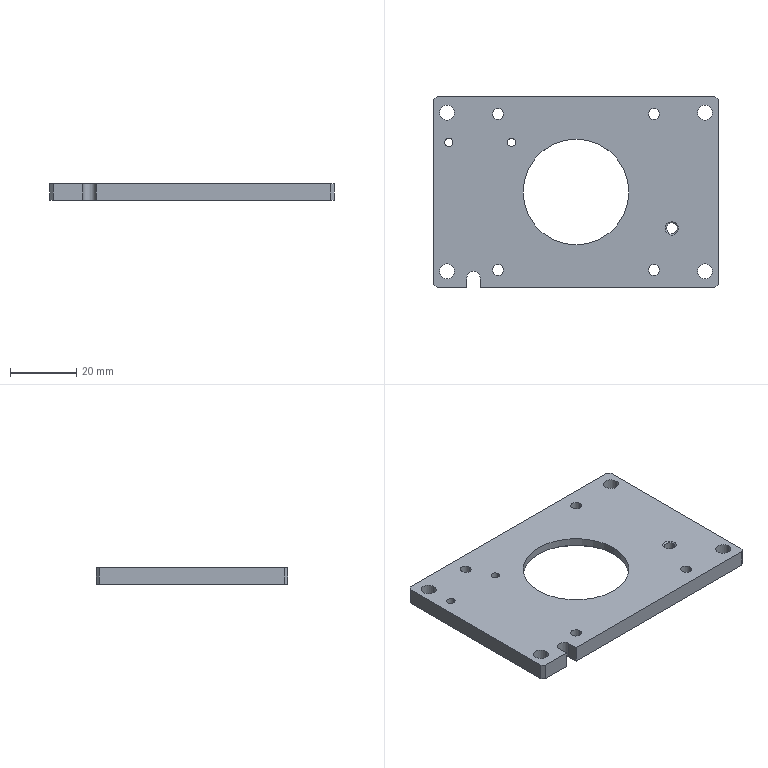Part | SolidWorks | features ICE 5, HoleWzd 4, 3DProfileFeature 2, MirrorPattern 2, Chamfer 1, Cut 1, Extrusion 1, LPattern 1 | 1 solid | 43 faces | box 86 x 58 x 5 mm | volume 19221 mm3 | cylinder 27 | plane 14 | cone 2 | commonest cylinder face diameters 3.3 x10 4.5 x8 2.5 x4 32 x2 39 x2 4 x1
STEP:
#1=CARTESIAN_POINT('',(27.35,-11.,4.625));
#2=VERTEX_POINT('',#1);
#3=CARTESIAN_POINT('',(30.65,-11.,4.625));
#4=VERTEX_POINT('',#3);
#5=CARTESIAN_POINT('',(29.,-11.,4.625));
#6=DIRECTION('',(0.,0.,1.));
#7=DIRECTION('',(1.,0.,0.));
#8=AXIS2_PLACEMENT_3D('',#5,#6,#7);
#9=CIRCLE('',#8,1.65);
#10=EDGE_CURVE('',#2,#4,#9,.T.);
#11=ORIENTED_EDGE('',*,*,#10,.F.);
#12=CARTESIAN_POINT('',(26.975,-11.,5.));
#13=VERTEX_POINT('',#12);
#14=CARTESIAN_POINT('',(26.975,-11.,5.));
#15=DIRECTION('',(-0.7071,0.,0.7071));
#16=VECTOR('',#15,1000.);
#17=LINE('',#14,#16);
#18=EDGE_CURVE('',#2,#13,#17,.T.);
#19=ORIENTED_EDGE('',*,*,#18,.T.);
#20=CARTESIAN_POINT('',(31.025,-11.,5.));
#21=VERTEX_POINT('',#20);
#22=CARTESIAN_POINT('',(29.,-11.,5.));
#23=DIRECTION('',(0.,0.,1.));
#24=DIRECTION('',(1.,0.,0.));
#25=AXIS2_PLACEMENT_3D('',#22,#23,#24);
#26=CIRCLE('',#25,2.025);
#27=EDGE_CURVE('',#13,#21,#26,.T.);
#28=ORIENTED_EDGE('',*,*,#27,.T.);
#29=CARTESIAN_POINT('',(31.025,-11.,5.));
#30=DIRECTION('',(0.7071,0.,0.7071));
#31=VECTOR('',#30,1000.);
#32=LINE('',#29,#31);
#33=EDGE_CURVE('',#4,#21,#32,.T.);
#34=ORIENTED_EDGE('',*,*,#33,.F.);
#35=EDGE_LOOP('',(#11,#19,#28,#34));
#36=FACE_OUTER_BOUND('',#35,.T.);
#37=CARTESIAN_POINT('',(29.,-11.,5.));
#38=DIRECTION('',(0.,0.,1.));
#39=DIRECTION('',(1.,0.,0.));
#40=AXIS2_PLACEMENT_3D('',#37,#38,#39);
#41=CONICAL_SURFACE('',#40,2.025,0.7854);
#42=ADVANCED_FACE('',(#36),#41,.F.);
#43=CARTESIAN_POINT('',(27.35,-11.,0.));
#44=VERTEX_POINT('',#43);
#45=CARTESIAN_POINT('',(30.65,-11.,0.));
#46=VERTEX_POINT('',#45);
#47=CARTESIAN_POINT('',(29.,-11.,0.));
#48=DIRECTION('',(0.,0.,1.));
#49=DIRECTION('',(1.,0.,0.));
#50=AXIS2_PLACEMENT_3D('',#47,#48,#49);
#51=CIRCLE('',#50,1.65);
#52=EDGE_CURVE('',#44,#46,#51,.T.);
#53=ORIENTED_EDGE('',*,*,#52,.F.);
#54=CARTESIAN_POINT('',(27.35,-11.,5.));
#55=DIRECTION('',(0.,0.,1.));
#56=VECTOR('',#55,1000.);
#57=LINE('',#54,#56);
#58=EDGE_CURVE('',#44,#2,#57,.T.);
#59=ORIENTED_EDGE('',*,*,#58,.T.);
#60=ORIENTED_EDGE('',*,*,#10,.T.);
#61=CARTESIAN_POINT('',(30.65,-11.,5.));
#62=DIRECTION('',(0.,0.,1.));
#63=VECTOR('',#62,1000.);
#64=LINE('',#61,#63);
#65=EDGE_CURVE('',#46,#4,#64,.T.);
#66=ORIENTED_EDGE('',*,*,#65,.F.);
#67=EDGE_LOOP('',(#53,#59,#60,#66));
#68=FACE_OUTER_BOUND('',#67,.T.);
#69=CARTESIAN_POINT('',(29.,-11.,5.));
#70=DIRECTION('',(0.,0.,1.));
#71=DIRECTION('',(1.,0.,0.));
#72=AXIS2_PLACEMENT_3D('',#69,#70,#71);
#73=CYLINDRICAL_SURFACE('',#72,1.65);
#74=ADVANCED_FACE('',(#68),#73,.F.);
#75=CARTESIAN_POINT('',(19.5,0.,2.6));
#76=VERTEX_POINT('',#75);
#77=CARTESIAN_POINT('',(-19.5,0.,2.6));
#78=VERTEX_POINT('',#77);
#79=CARTESIAN_POINT('',(0.,0.,2.6));
#80=DIRECTION('',(0.,0.,-1.));
#81=DIRECTION('',(-1.,0.,0.));
#82=AXIS2_PLACEMENT_3D('',#79,#80,#81);
#83=CIRCLE('',#82,19.5);
#84=EDGE_CURVE('',#76,#78,#83,.T.);
#85=ORIENTED_EDGE('',*,*,#84,.F.);
#86=CARTESIAN_POINT('',(19.5,0.,0.));
#87=VERTEX_POINT('',#86);
#88=CARTESIAN_POINT('',(19.5,0.,2.6));
#89=DIRECTION('',(0.,0.,-1.));
#90=VECTOR('',#89,1000.);
#91=LINE('',#88,#90);
#92=EDGE_CURVE('',#76,#87,#91,.T.);
#93=ORIENTED_EDGE('',*,*,#92,.T.);
#94=CARTESIAN_POINT('',(-19.5,0.,0.));
#95=VERTEX_POINT('',#94);
#96=CARTESIAN_POINT('',(0.,0.,0.));
#97=DIRECTION('',(0.,0.,-1.));
#98=DIRECTION('',(-1.,0.,0.));
#99=AXIS2_PLACEMENT_3D('',#96,#97,#98);
#100=CIRCLE('',#99,19.5);
#101=EDGE_CURVE('',#87,#95,#100,.T.);
#102=ORIENTED_EDGE('',*,*,#101,.T.);
#103=CARTESIAN_POINT('',(-19.5,0.,2.6));
#104=DIRECTION('',(0.,0.,-1.));
#105=VECTOR('',#104,1000.);
#106=LINE('',#103,#105);
#107=EDGE_CURVE('',#78,#95,#106,.T.);
#108=ORIENTED_EDGE('',*,*,#107,.F.);
#109=EDGE_LOOP('',(#85,#93,#102,#108));
#110=FACE_OUTER_BOUND('',#109,.T.);
#111=CARTESIAN_POINT('',(0.,0.,2.6));
#112=DIRECTION('',(0.,0.,-1.));
#113=DIRECTION('',(-1.,0.,0.));
#114=AXIS2_PLACEMENT_3D('',#111,#112,#113);
#115=CYLINDRICAL_SURFACE('',#114,19.5);
#116=ADVANCED_FACE('',(#110),#115,.F.);
#117=CARTESIAN_POINT('',(25.22,-23.57,0.));
#118=VERTEX_POINT('',#117);
#119=CARTESIAN_POINT('',(21.92,-23.57,0.));
#120=VERTEX_POINT('',#119);
#121=CARTESIAN_POINT('',(23.57,-23.57,0.));
#122=DIRECTION('',(0.,0.,-1.));
#123=DIRECTION('',(1.,0.,0.));
#124=AXIS2_PLACEMENT_3D('',#121,#122,#123);
#125=CIRCLE('',#124,1.65);
#126=EDGE_CURVE('',#118,#120,#125,.T.);
#127=ORIENTED_EDGE('',*,*,#126,.T.);
#128=CARTESIAN_POINT('',(21.92,-23.57,5.));
#129=VERTEX_POINT('',#128);
#130=CARTESIAN_POINT('',(21.92,-23.57,5.));
#131=DIRECTION('',(0.,0.,1.));
#132=VECTOR('',#131,1000.);
#133=LINE('',#130,#132);
#134=EDGE_CURVE('',#120,#129,#133,.T.);
#135=ORIENTED_EDGE('',*,*,#134,.T.);
#136=CARTESIAN_POINT('',(25.22,-23.57,5.));
#137=VERTEX_POINT('',#136);
#138=CARTESIAN_POINT('',(23.57,-23.57,5.));
#139=DIRECTION('',(0.,0.,1.));
#140=DIRECTION('',(1.,0.,0.));
#141=AXIS2_PLACEMENT_3D('',#138,#139,#140);
#142=CIRCLE('',#141,1.65);
#143=EDGE_CURVE('',#129,#137,#142,.T.);
#144=ORIENTED_EDGE('',*,*,#143,.T.);
#145=CARTESIAN_POINT('',(25.22,-23.57,5.));
#146=DIRECTION('',(0.,0.,1.));
#147=VECTOR('',#146,1000.);
#148=LINE('',#145,#147);
#149=EDGE_CURVE('',#118,#137,#148,.T.);
#150=ORIENTED_EDGE('',*,*,#149,.F.);
#151=EDGE_LOOP('',(#127,#135,#144,#150));
#152=FACE_OUTER_BOUND('',#151,.T.);
#153=CARTESIAN_POINT('',(23.57,-23.57,5.));
#154=DIRECTION('',(0.,0.,1.));
#155=DIRECTION('',(1.,0.,0.));
#156=AXIS2_PLACEMENT_3D('',#153,#154,#155);
#157=CYLINDRICAL_SURFACE('',#156,1.65);
#158=ADVANCED_FACE('',(#152),#157,.F.);
#159=CARTESIAN_POINT('',(25.22,23.57,0.));
#160=VERTEX_POINT('',#159);
#161=CARTESIAN_POINT('',(21.92,23.57,0.));
#162=VERTEX_POINT('',#161);
#163=CARTESIAN_POINT('',(23.57,23.57,0.));
#164=DIRECTION('',(0.,0.,-1.));
#165=DIRECTION('',(1.,0.,0.));
#166=AXIS2_PLACEMENT_3D('',#163,#164,#165);
#167=CIRCLE('',#166,1.65);
#168=EDGE_CURVE('',#160,#162,#167,.T.);
#169=ORIENTED_EDGE('',*,*,#168,.T.);
#170=CARTESIAN_POINT('',(21.92,23.57,5.));
#171=VERTEX_POINT('',#170);
#172=CARTESIAN_POINT('',(21.92,23.57,5.));
#173=DIRECTION('',(0.,0.,1.));
#174=VECTOR('',#173,1000.);
#175=LINE('',#172,#174);
#176=EDGE_CURVE('',#162,#171,#175,.T.);
#177=ORIENTED_EDGE('',*,*,#176,.T.);
#178=CARTESIAN_POINT('',(25.22,23.57,5.));
#179=VERTEX_POINT('',#178);
#180=CARTESIAN_POINT('',(23.57,23.57,5.));
#181=DIRECTION('',(0.,0.,1.));
#182=DIRECTION('',(1.,0.,0.));
#183=AXIS2_PLACEMENT_3D('',#180,#181,#182);
#184=CIRCLE('',#183,1.65);
#185=EDGE_CURVE('',#171,#179,#184,.T.);
#186=ORIENTED_EDGE('',*,*,#185,.T.);
#187=CARTESIAN_POINT('',(25.22,23.57,5.));
#188=DIRECTION('',(0.,0.,1.));
#189=VECTOR('',#188,1000.);
#190=LINE('',#187,#189);
#191=EDGE_CURVE('',#160,#179,#190,.T.);
#192=ORIENTED_EDGE('',*,*,#191,.F.);
#193=EDGE_LOOP('',(#169,#177,#186,#192));
#194=FACE_OUTER_BOUND('',#193,.T.);
#195=CARTESIAN_POINT('',(23.57,23.57,5.));
#196=DIRECTION('',(0.,0.,1.));
#197=DIRECTION('',(1.,0.,0.));
#198=AXIS2_PLACEMENT_3D('',#195,#196,#197);
#199=CYLINDRICAL_SURFACE('',#198,1.65);
#200=ADVANCED_FACE('',(#194),#199,.F.);
#201=CARTESIAN_POINT('',(-21.92,-23.57,0.));
#202=VERTEX_POINT('',#201);
#203=CARTESIAN_POINT('',(-25.22,-23.57,0.));
#204=VERTEX_POINT('',#203);
#205=CARTESIAN_POINT('',(-23.57,-23.57,0.));
#206=DIRECTION('',(0.,0.,-1.));
#207=DIRECTION('',(1.,0.,0.));
#208=AXIS2_PLACEMENT_3D('',#205,#206,#207);
#209=CIRCLE('',#208,1.65);
#210=EDGE_CURVE('',#202,#204,#209,.T.);
#211=ORIENTED_EDGE('',*,*,#210,.T.);
#212=CARTESIAN_POINT('',(-25.22,-23.57,5.));
#213=VERTEX_POINT('',#212);
#214=CARTESIAN_POINT('',(-25.22,-23.57,5.));
#215=DIRECTION('',(0.,0.,1.));
#216=VECTOR('',#215,1000.);
#217=LINE('',#214,#216);
#218=EDGE_CURVE('',#204,#213,#217,.T.);
#219=ORIENTED_EDGE('',*,*,#218,.T.);
#220=CARTESIAN_POINT('',(-21.92,-23.57,5.));
#221=VERTEX_POINT('',#220);
#222=CARTESIAN_POINT('',(-23.57,-23.57,5.));
#223=DIRECTION('',(0.,0.,1.));
#224=DIRECTION('',(1.,0.,0.));
#225=AXIS2_PLACEMENT_3D('',#222,#223,#224);
#226=CIRCLE('',#225,1.65);
#227=EDGE_CURVE('',#213,#221,#226,.T.);
#228=ORIENTED_EDGE('',*,*,#227,.T.);
#229=CARTESIAN_POINT('',(-21.92,-23.57,5.));
#230=DIRECTION('',(0.,0.,1.));
#231=VECTOR('',#230,1000.);
#232=LINE('',#229,#231);
#233=EDGE_CURVE('',#202,#221,#232,.T.);
#234=ORIENTED_EDGE('',*,*,#233,.F.);
#235=EDGE_LOOP('',(#211,#219,#228,#234));
#236=FACE_OUTER_BOUND('',#235,.T.);
#237=CARTESIAN_POINT('',(-23.57,-23.57,5.));
#238=DIRECTION('',(0.,0.,1.));
#239=DIRECTION('',(1.,0.,0.));
#240=AXIS2_PLACEMENT_3D('',#237,#238,#239);
#241=CYLINDRICAL_SURFACE('',#240,1.65);
#242=ADVANCED_FACE('',(#236),#241,.F.);
#243=CARTESIAN_POINT('',(-21.92,23.57,0.));
#244=VERTEX_POINT('',#243);
#245=CARTESIAN_POINT('',(-25.22,23.57,0.));
#246=VERTEX_POINT('',#245);
#247=CARTESIAN_POINT('',(-23.57,23.57,0.));
#248=DIRECTION('',(0.,0.,-1.));
#249=DIRECTION('',(1.,0.,0.));
#250=AXIS2_PLACEMENT_3D('',#247,#248,#249);
#251=CIRCLE('',#250,1.65);
#252=EDGE_CURVE('',#244,#246,#251,.T.);
#253=ORIENTED_EDGE('',*,*,#252,.T.);
#254=CARTESIAN_POINT('',(-25.22,23.57,5.));
#255=VERTEX_POINT('',#254);
#256=CARTESIAN_POINT('',(-25.22,23.57,5.));
#257=DIRECTION('',(0.,0.,1.));
#258=VECTOR('',#257,1000.);
#259=LINE('',#256,#258);
#260=EDGE_CURVE('',#246,#255,#259,.T.);
#261=ORIENTED_EDGE('',*,*,#260,.T.);
#262=CARTESIAN_POINT('',(-21.92,23.57,5.));
#263=VERTEX_POINT('',#262);
#264=CARTESIAN_POINT('',(-23.57,23.57,5.));
#265=DIRECTION('',(0.,0.,1.));
#266=DIRECTION('',(1.,0.,0.));
#267=AXIS2_PLACEMENT_3D('',#264,#265,#266);
#268=CIRCLE('',#267,1.65);
#269=EDGE_CURVE('',#255,#263,#268,.T.);
#270=ORIENTED_EDGE('',*,*,#269,.T.);
#271=CARTESIAN_POINT('',(-21.92,23.57,5.));
#272=DIRECTION('',(0.,0.,1.));
#273=VECTOR('',#272,1000.);
#274=LINE('',#271,#273);
#275=EDGE_CURVE('',#244,#263,#274,.T.);
#276=ORIENTED_EDGE('',*,*,#275,.F.);
#277=EDGE_LOOP('',(#253,#261,#270,#276));
#278=FACE_OUTER_BOUND('',#277,.T.);
#279=CARTESIAN_POINT('',(-23.57,23.57,5.));
#280=DIRECTION('',(0.,0.,1.));
#281=DIRECTION('',(1.,0.,0.));
#282=AXIS2_PLACEMENT_3D('',#279,#280,#281);
#283=CYLINDRICAL_SURFACE('',#282,1.65);
#284=ADVANCED_FACE('',(#278),#283,.F.);
#285=CARTESIAN_POINT('',(-37.25,15.,0.));
#286=VERTEX_POINT('',#285);
#287=CARTESIAN_POINT('',(-39.75,15.,0.));
#288=VERTEX_POINT('',#287);
#289=CARTESIAN_POINT('',(-38.5,15.,0.));
#290=DIRECTION('',(0.,0.,-1.));
#291=DIRECTION('',(1.,0.,0.));
#292=AXIS2_PLACEMENT_3D('',#289,#290,#291);
#293=CIRCLE('',#292,1.25);
#294=EDGE_CURVE('',#286,#288,#293,.T.);
#295=ORIENTED_EDGE('',*,*,#294,.T.);
#296=CARTESIAN_POINT('',(-39.75,15.,5.));
#297=VERTEX_POINT('',#296);
#298=CARTESIAN_POINT('',(-39.75,15.,5.));
#299=DIRECTION('',(0.,0.,1.));
#300=VECTOR('',#299,1000.);
#301=LINE('',#298,#300);
#302=EDGE_CURVE('',#288,#297,#301,.T.);
#303=ORIENTED_EDGE('',*,*,#302,.T.);
#304=CARTESIAN_POINT('',(-37.25,15.,5.));
#305=VERTEX_POINT('',#304);
#306=CARTESIAN_POINT('',(-38.5,15.,5.));
#307=DIRECTION('',(0.,0.,1.));
#308=DIRECTION('',(1.,0.,0.));
#309=AXIS2_PLACEMENT_3D('',#306,#307,#308);
#310=CIRCLE('',#309,1.25);
#311=EDGE_CURVE('',#297,#305,#310,.T.);
#312=ORIENTED_EDGE('',*,*,#311,.T.);
#313=CARTESIAN_POINT('',(-37.25,15.,5.));
#314=DIRECTION('',(0.,0.,1.));
#315=VECTOR('',#314,1000.);
#316=LINE('',#313,#315);
#317=EDGE_CURVE('',#286,#305,#316,.T.);
#318=ORIENTED_EDGE('',*,*,#317,.F.);
#319=EDGE_LOOP('',(#295,#303,#312,#318));
#320=FACE_OUTER_BOUND('',#319,.T.);
#321=CARTESIAN_POINT('',(-38.5,15.,5.));
#322=DIRECTION('',(0.,0.,1.));
#323=DIRECTION('',(1.,0.,0.));
#324=AXIS2_PLACEMENT_3D('',#321,#322,#323);
#325=CYLINDRICAL_SURFACE('',#324,1.25);
#326=ADVANCED_FACE('',(#320),#325,.F.);
#327=CARTESIAN_POINT('',(-18.25,15.,0.));
#328=VERTEX_POINT('',#327);
#329=CARTESIAN_POINT('',(-20.75,15.,0.));
#330=VERTEX_POINT('',#329);
#331=CARTESIAN_POINT('',(-19.5,15.,0.));
#332=DIRECTION('',(0.,0.,-1.));
#333=DIRECTION('',(1.,0.,0.));
#334=AXIS2_PLACEMENT_3D('',#331,#332,#333);
#335=CIRCLE('',#334,1.25);
#336=EDGE_CURVE('',#328,#330,#335,.T.);
#337=ORIENTED_EDGE('',*,*,#336,.T.);
#338=CARTESIAN_POINT('',(-20.75,15.,5.));
#339=VERTEX_POINT('',#338);
#340=CARTESIAN_POINT('',(-20.75,15.,5.));
#341=DIRECTION('',(0.,0.,1.));
#342=VECTOR('',#341,1000.);
#343=LINE('',#340,#342);
#344=EDGE_CURVE('',#330,#339,#343,.T.);
#345=ORIENTED_EDGE('',*,*,#344,.T.);
#346=CARTESIAN_POINT('',(-18.25,15.,5.));
#347=VERTEX_POINT('',#346);
#348=CARTESIAN_POINT('',(-19.5,15.,5.));
#349=DIRECTION('',(0.,0.,1.));
#350=DIRECTION('',(1.,0.,0.));
#351=AXIS2_PLACEMENT_3D('',#348,#349,#350);
#352=CIRCLE('',#351,1.25);
#353=EDGE_CURVE('',#339,#347,#352,.T.);
#354=ORIENTED_EDGE('',*,*,#353,.T.);
#355=CARTESIAN_POINT('',(-18.25,15.,5.));
#356=DIRECTION('',(0.,0.,1.));
#357=VECTOR('',#356,1000.);
#358=LINE('',#355,#357);
#359=EDGE_CURVE('',#328,#347,#358,.T.);
#360=ORIENTED_EDGE('',*,*,#359,.F.);
#361=EDGE_LOOP('',(#337,#345,#354,#360));
#362=FACE_OUTER_BOUND('',#361,.T.);
#363=CARTESIAN_POINT('',(-19.5,15.,5.));
#364=DIRECTION('',(0.,0.,1.));
#365=DIRECTION('',(1.,0.,0.));
#366=AXIS2_PLACEMENT_3D('',#363,#364,#365);
#367=CYLINDRICAL_SURFACE('',#366,1.25);
#368=ADVANCED_FACE('',(#362),#367,.F.);
#369=CARTESIAN_POINT('',(-41.25,-24.,5.));
#370=VERTEX_POINT('',#369);
#371=CARTESIAN_POINT('',(-36.75,-24.,5.));
#372=VERTEX_POINT('',#371);
#373=CARTESIAN_POINT('',(-39.,-24.,5.));
#374=DIRECTION('',(0.,0.,1.));
#375=DIRECTION('',(-1.,0.,0.));
#376=AXIS2_PLACEMENT_3D('',#373,#374,#375);
#377=CIRCLE('',#376,2.25);
#378=EDGE_CURVE('',#370,#372,#377,.T.);
#379=ORIENTED_EDGE('',*,*,#378,.T.);
#380=CARTESIAN_POINT('',(-36.75,-24.,0.));
#381=VERTEX_POINT('',#380);
#382=CARTESIAN_POINT('',(-36.75,-24.,5.));
#383=DIRECTION('',(0.,0.,-1.));
#384=VECTOR('',#383,1000.);
#385=LINE('',#382,#384);
#386=EDGE_CURVE('',#372,#381,#385,.T.);
#387=ORIENTED_EDGE('',*,*,#386,.T.);
#388=CARTESIAN_POINT('',(-41.25,-24.,0.));
#389=VERTEX_POINT('',#388);
#390=CARTESIAN_POINT('',(-39.,-24.,0.));
#391=DIRECTION('',(0.,0.,1.));
#392=DIRECTION('',(1.,0.,0.));
#393=AXIS2_PLACEMENT_3D('',#390,#391,#392);
#394=CIRCLE('',#393,2.25);
#395=EDGE_CURVE('',#389,#381,#394,.T.);
#396=ORIENTED_EDGE('',*,*,#395,.F.);
#397=CARTESIAN_POINT('',(-41.25,-24.,5.));
#398=DIRECTION('',(0.,0.,-1.));
#399=VECTOR('',#398,1000.);
#400=LINE('',#397,#399);
#401=EDGE_CURVE('',#370,#389,#400,.T.);
#402=ORIENTED_EDGE('',*,*,#401,.F.);
#403=EDGE_LOOP('',(#379,#387,#396,#402));
#404=FACE_OUTER_BOUND('',#403,.T.);
#405=CARTESIAN_POINT('',(-39.,-24.,5.));
#406=DIRECTION('',(0.,0.,-1.));
#407=DIRECTION('',(-1.,0.,0.));
#408=AXIS2_PLACEMENT_3D('',#405,#406,#407);
#409=CYLINDRICAL_SURFACE('',#408,2.25);
#410=ADVANCED_FACE('',(#404),#409,.F.);
#411=CARTESIAN_POINT('',(36.75,-24.,5.));
#412=VERTEX_POINT('',#411);
#413=CARTESIAN_POINT('',(41.25,-24.,5.));
#414=VERTEX_POINT('',#413);
#415=CARTESIAN_POINT('',(39.,-24.,5.));
#416=DIRECTION('',(0.,0.,1.));
#417=DIRECTION('',(1.,0.,0.));
#418=AXIS2_PLACEMENT_3D('',#415,#416,#417);
#419=CIRCLE('',#418,2.25);
#420=EDGE_CURVE('',#412,#414,#419,.T.);
#421=ORIENTED_EDGE('',*,*,#420,.T.);
#422=CARTESIAN_POINT('',(41.25,-24.,0.));
#423=VERTEX_POINT('',#422);
#424=CARTESIAN_POINT('',(41.25,-24.,5.));
#425=DIRECTION('',(0.,0.,-1.));
#426=VECTOR('',#425,1000.);
#427=LINE('',#424,#426);
#428=EDGE_CURVE('',#414,#423,#427,.T.);
#429=ORIENTED_EDGE('',*,*,#428,.T.);
#430=CARTESIAN_POINT('',(36.75,-24.,0.));
#431=VERTEX_POINT('',#430);
#432=CARTESIAN_POINT('',(39.,-24.,0.));
#433=DIRECTION('',(0.,0.,1.));
#434=DIRECTION('',(1.,0.,0.));
#435=AXIS2_PLACEMENT_3D('',#432,#433,#434);
#436=CIRCLE('',#435,2.25);
#437=EDGE_CURVE('',#431,#423,#436,.T.);
#438=ORIENTED_EDGE('',*,*,#437,.F.);
#439=CARTESIAN_POINT('',(36.75,-24.,5.));
#440=DIRECTION('',(0.,0.,-1.));
#441=VECTOR('',#440,1000.);
#442=LINE('',#439,#441);
#443=EDGE_CURVE('',#412,#431,#442,.T.);
#444=ORIENTED_EDGE('',*,*,#443,.F.);
#445=EDGE_LOOP('',(#421,#429,#438,#444));
#446=FACE_OUTER_BOUND('',#445,.T.);
#447=CARTESIAN_POINT('',(39.,-24.,5.));
#448=DIRECTION('',(0.,0.,-1.));
#449=DIRECTION('',(-1.,0.,0.));
#450=AXIS2_PLACEMENT_3D('',#447,#448,#449);
#451=CYLINDRICAL_SURFACE('',#450,2.25);
#452=ADVANCED_FACE('',(#446),#451,.F.);
#453=CARTESIAN_POINT('',(36.75,24.,5.));
#454=VERTEX_POINT('',#453);
#455=CARTESIAN_POINT('',(41.25,24.,5.));
#456=VERTEX_POINT('',#455);
#457=CARTESIAN_POINT('',(39.,24.,5.));
#458=DIRECTION('',(0.,0.,1.));
#459=DIRECTION('',(-1.,0.,0.));
#460=AXIS2_PLACEMENT_3D('',#457,#458,#459);
#461=CIRCLE('',#460,2.25);
#462=EDGE_CURVE('',#454,#456,#461,.T.);
#463=ORIENTED_EDGE('',*,*,#462,.T.);
#464=CARTESIAN_POINT('',(41.25,24.,0.));
#465=VERTEX_POINT('',#464);
#466=CARTESIAN_POINT('',(41.25,24.,5.));
#467=DIRECTION('',(0.,0.,-1.));
#468=VECTOR('',#467,1000.);
#469=LINE('',#466,#468);
#470=EDGE_CURVE('',#456,#465,#469,.T.);
#471=ORIENTED_EDGE('',*,*,#470,.T.);
#472=CARTESIAN_POINT('',(36.75,24.,0.));
#473=VERTEX_POINT('',#472);
#474=CARTESIAN_POINT('',(39.,24.,0.));
#475=DIRECTION('',(0.,0.,1.));
#476=DIRECTION('',(1.,0.,0.));
#477=AXIS2_PLACEMENT_3D('',#474,#475,#476);
#478=CIRCLE('',#477,2.25);
#479=EDGE_CURVE('',#473,#465,#478,.T.);
#480=ORIENTED_EDGE('',*,*,#479,.F.);
#481=CARTESIAN_POINT('',(36.75,24.,5.));
#482=DIRECTION('',(0.,0.,-1.));
#483=VECTOR('',#482,1000.);
#484=LINE('',#481,#483);
#485=EDGE_CURVE('',#454,#473,#484,.T.);
#486=ORIENTED_EDGE('',*,*,#485,.F.);
#487=EDGE_LOOP('',(#463,#471,#480,#486));
#488=FACE_OUTER_BOUND('',#487,.T.);
#489=CARTESIAN_POINT('',(39.,24.,5.));
#490=DIRECTION('',(0.,0.,-1.));
#491=DIRECTION('',(-1.,0.,0.));
#492=AXIS2_PLACEMENT_3D('',#489,#490,#491);
#493=CYLINDRICAL_SURFACE('',#492,2.25);
#494=ADVANCED_FACE('',(#488),#493,.F.);
#495=CARTESIAN_POINT('',(-41.25,24.,5.));
#496=VERTEX_POINT('',#495);
#497=CARTESIAN_POINT('',(-36.75,24.,5.));
#498=VERTEX_POINT('',#497);
#499=CARTESIAN_POINT('',(-39.,24.,5.));
#500=DIRECTION('',(0.,0.,1.));
#501=DIRECTION('',(1.,0.,0.));
#502=AXIS2_PLACEMENT_3D('',#499,#500,#501);
#503=CIRCLE('',#502,2.25);
#504=EDGE_CURVE('',#496,#498,#503,.T.);
#505=ORIENTED_EDGE('',*,*,#504,.T.);
#506=CARTESIAN_POINT('',(-36.75,24.,0.));
#507=VERTEX_POINT('',#506);
#508=CARTESIAN_POINT('',(-36.75,24.,5.));
#509=DIRECTION('',(0.,0.,-1.));
#510=VECTOR('',#509,1000.);
#511=LINE('',#508,#510);
#512=EDGE_CURVE('',#498,#507,#511,.T.);
#513=ORIENTED_EDGE('',*,*,#512,.T.);
#514=CARTESIAN_POINT('',(-41.25,24.,0.));
#515=VERTEX_POINT('',#514);
#516=CARTESIAN_POINT('',(-39.,24.,0.));
#517=DIRECTION('',(0.,0.,1.));
#518=DIRECTION('',(1.,0.,0.));
#519=AXIS2_PLACEMENT_3D('',#516,#517,#518);
#520=CIRCLE('',#519,2.25);
#521=EDGE_CURVE('',#515,#507,#520,.T.);
#522=ORIENTED_EDGE('',*,*,#521,.F.);
#523=CARTESIAN_POINT('',(-41.25,24.,5.));
#524=DIRECTION('',(0.,0.,-1.));
#525=VECTOR('',#524,1000.);
#526=LINE('',#523,#525);
#527=EDGE_CURVE('',#496,#515,#526,.T.);
#528=ORIENTED_EDGE('',*,*,#527,.F.);
#529=EDGE_LOOP('',(#505,#513,#522,#528));
#530=FACE_OUTER_BOUND('',#529,.T.);
#531=CARTESIAN_POINT('',(-39.,24.,5.));
#532=DIRECTION('',(0.,0.,-1.));
#533=DIRECTION('',(-1.,0.,0.));
#534=AXIS2_PLACEMENT_3D('',#531,#532,#533);
#535=CYLINDRICAL_SURFACE('',#534,2.25);
#536=ADVANCED_FACE('',(#530),#535,.F.);
#537=CARTESIAN_POINT('',(-16.,0.,5.));
#538=VERTEX_POINT('',#537);
#539=CARTESIAN_POINT('',(16.,0.,5.));
#540=VERTEX_POINT('',#539);
#541=CARTESIAN_POINT('',(0.,0.,5.));
#542=DIRECTION('',(0.,0.,1.));
#543=DIRECTION('',(1.,0.,0.));
#544=AXIS2_PLACEMENT_3D('',#541,#542,#543);
#545=CIRCLE('',#544,16.);
#546=EDGE_CURVE('',#538,#540,#545,.T.);
#547=ORIENTED_EDGE('',*,*,#546,.T.);
#548=CARTESIAN_POINT('',(16.,0.,2.6));
#549=VERTEX_POINT('',#548);
#550=CARTESIAN_POINT('',(16.,0.,5.));
#551=DIRECTION('',(0.,0.,-1.));
#552=VECTOR('',#551,1000.);
#553=LINE('',#550,#552);
#554=EDGE_CURVE('',#540,#549,#553,.T.);
#555=ORIENTED_EDGE('',*,*,#554,.T.);
#556=CARTESIAN_POINT('',(-16.,0.,2.6));
#557=VERTEX_POINT('',#556);
#558=CARTESIAN_POINT('',(0.,0.,2.6));
#559=DIRECTION('',(0.,0.,-1.));
#560=DIRECTION('',(-1.,0.,0.));
#561=AXIS2_PLACEMENT_3D('',#558,#559,#560);
#562=CIRCLE('',#561,16.);
#563=EDGE_CURVE('',#549,#557,#562,.T.);
#564=ORIENTED_EDGE('',*,*,#563,.T.);
#565=CARTESIAN_POINT('',(-16.,0.,5.));
#566=DIRECTION('',(0.,0.,-1.));
#567=VECTOR('',#566,1000.);
#568=LINE('',#565,#567);
#569=EDGE_CURVE('',#538,#557,#568,.T.);
#570=ORIENTED_EDGE('',*,*,#569,.F.);
#571=EDGE_LOOP('',(#547,#555,#564,#570));
#572=FACE_OUTER_BOUND('',#571,.T.);
#573=CARTESIAN_POINT('',(0.,0.,5.));
#574=DIRECTION('',(0.,0.,-1.));
#575=DIRECTION('',(-1.,0.,0.));
#576=AXIS2_PLACEMENT_3D('',#573,#574,#575);
#577=CYLINDRICAL_SURFACE('',#576,16.);
#578=ADVANCED_FACE('',(#572),#577,.F.);
#579=ORIENTED_EDGE('',*,*,#554,.F.);
#580=CARTESIAN_POINT('',(0.,0.,5.));
#581=DIRECTION('',(0.,0.,1.));
#582=DIRECTION('',(1.,0.,0.));
#583=AXIS2_PLACEMENT_3D('',#580,#581,#582);
#584=CIRCLE('',#583,16.);
#585=EDGE_CURVE('',#540,#538,#584,.T.);
#586=ORIENTED_EDGE('',*,*,#585,.T.);
#587=ORIENTED_EDGE('',*,*,#569,.T.);
#588=CARTESIAN_POINT('',(0.,0.,2.6));
#589=DIRECTION('',(0.,0.,-1.));
#590=DIRECTION('',(-1.,0.,0.));
#591=AXIS2_PLACEMENT_3D('',#588,#589,#590);
#592=CIRCLE('',#591,16.);
#593=EDGE_CURVE('',#557,#549,#592,.T.);
#594=ORIENTED_EDGE('',*,*,#593,.T.);
#595=EDGE_LOOP('',(#579,#586,#587,#594));
#596=FACE_OUTER_BOUND('',#595,.T.);
#597=CARTESIAN_POINT('',(0.,0.,5.));
#598=DIRECTION('',(0.,0.,-1.));
#599=DIRECTION('',(-1.,0.,0.));
#600=AXIS2_PLACEMENT_3D('',#597,#598,#599);
#601=CYLINDRICAL_SURFACE('',#600,16.);
#602=ADVANCED_FACE('',(#596),#601,.F.);
#603=CARTESIAN_POINT('',(-42.,-29.,5.));
#604=VERTEX_POINT('',#603);
#605=CARTESIAN_POINT('',(-42.,-29.,0.));
#606=VERTEX_POINT('',#605);
#607=CARTESIAN_POINT('',(-42.,-29.,5.));
#608=DIRECTION('',(0.,0.,-1.));
#609=VECTOR('',#608,1000.);
#610=LINE('',#607,#609);
#611=EDGE_CURVE('',#604,#606,#610,.T.);
#612=ORIENTED_EDGE('',*,*,#611,.T.);
#613=CARTESIAN_POINT('',(-33.,-29.,0.));
#614=VERTEX_POINT('',#613);
#615=CARTESIAN_POINT('',(160.212,-29.,0.));
#616=DIRECTION('',(1.,0.,0.));
#617=VECTOR('',#616,1000.);
#618=LINE('',#615,#617);
#619=EDGE_CURVE('',#606,#614,#618,.T.);
#620=ORIENTED_EDGE('',*,*,#619,.T.);
#621=CARTESIAN_POINT('',(-33.,-29.,5.));
#622=VERTEX_POINT('',#621);
#623=CARTESIAN_POINT('',(-33.,-29.,-5.));
#624=DIRECTION('',(0.,0.,1.));
#625=VECTOR('',#624,1000.);
#626=LINE('',#623,#625);
#627=EDGE_CURVE('',#614,#622,#626,.T.);
#628=ORIENTED_EDGE('',*,*,#627,.T.);
#629=CARTESIAN_POINT('',(-43.,-29.,5.));
#630=DIRECTION('',(1.,0.,0.));
#631=VECTOR('',#630,1000.);
#632=LINE('',#629,#631);
#633=EDGE_CURVE('',#604,#622,#632,.T.);
#634=ORIENTED_EDGE('',*,*,#633,.F.);
#635=EDGE_LOOP('',(#612,#620,#628,#634));
#636=FACE_OUTER_BOUND('',#635,.T.);
#637=CARTESIAN_POINT('',(-43.,-29.,5.));
#638=DIRECTION('',(0.,1.,0.));
#639=DIRECTION('',(0.,0.,1.));
#640=AXIS2_PLACEMENT_3D('',#637,#638,#639);
#641=PLANE('',#640);
#642=ADVANCED_FACE('',(#636),#641,.F.);
#643=CARTESIAN_POINT('',(29.,-11.,5.));
#644=DIRECTION('',(0.,0.,1.));
#645=DIRECTION('',(1.,0.,0.));
#646=AXIS2_PLACEMENT_3D('',#643,#644,#645);
#647=CIRCLE('',#646,2.025);
#648=EDGE_CURVE('',#21,#13,#647,.T.);
#649=ORIENTED_EDGE('',*,*,#648,.F.);
#650=ORIENTED_EDGE('',*,*,#27,.F.);
#651=EDGE_LOOP('',(#649,#650));
#652=FACE_BOUND('',#651,.T.);
#653=CARTESIAN_POINT('',(-29.,-29.,5.));
#654=VERTEX_POINT('',#653);
#655=CARTESIAN_POINT('',(42.,-29.,5.));
#656=VERTEX_POINT('',#655);
#657=CARTESIAN_POINT('',(-43.,-29.,5.));
#658=DIRECTION('',(1.,0.,0.));
#659=VECTOR('',#658,1000.);
#660=LINE('',#657,#659);
#661=EDGE_CURVE('',#654,#656,#660,.T.);
#662=ORIENTED_EDGE('',*,*,#661,.T.);
#663=CARTESIAN_POINT('',(43.,-28.,5.));
#664=VERTEX_POINT('',#663);
#665=CARTESIAN_POINT('',(35.5,-35.5,5.));
#666=DIRECTION('',(0.7071,0.7071,0.));
#667=VECTOR('',#666,1000.);
#668=LINE('',#665,#667);
#669=EDGE_CURVE('',#656,#664,#668,.T.);
#670=ORIENTED_EDGE('',*,*,#669,.T.);
#671=CARTESIAN_POINT('',(43.,28.,5.));
#672=VERTEX_POINT('',#671);
#673=CARTESIAN_POINT('',(43.,29.,5.));
#674=DIRECTION('',(0.,1.,0.));
#675=VECTOR('',#674,1000.);
#676=LINE('',#673,#675);
#677=EDGE_CURVE('',#664,#672,#676,.T.);
#678=ORIENTED_EDGE('',*,*,#677,.T.);
#679=CARTESIAN_POINT('',(42.,29.,5.));
#680=VERTEX_POINT('',#679);
#681=CARTESIAN_POINT('',(35.5,35.5,5.));
#682=DIRECTION('',(-0.7071,0.7071,0.));
#683=VECTOR('',#682,1000.);
#684=LINE('',#681,#683);
#685=EDGE_CURVE('',#672,#680,#684,.T.);
#686=ORIENTED_EDGE('',*,*,#685,.T.);
#687=CARTESIAN_POINT('',(-42.,29.,5.));
#688=VERTEX_POINT('',#687);
#689=CARTESIAN_POINT('',(-43.,29.,5.));
#690=DIRECTION('',(-1.,0.,0.));
#691=VECTOR('',#690,1000.);
#692=LINE('',#689,#691);
#693=EDGE_CURVE('',#680,#688,#692,.T.);
#694=ORIENTED_EDGE('',*,*,#693,.T.);
#695=CARTESIAN_POINT('',(-43.,28.,5.));
#696=VERTEX_POINT('',#695);
#697=CARTESIAN_POINT('',(-35.5,35.5,5.));
#698=DIRECTION('',(-0.7071,-0.7071,0.));
#699=VECTOR('',#698,1000.);
#700=LINE('',#697,#699);
#701=EDGE_CURVE('',#688,#696,#700,.T.);
#702=ORIENTED_EDGE('',*,*,#701,.T.);
#703=CARTESIAN_POINT('',(-43.,-28.,5.));
#704=VERTEX_POINT('',#703);
#705=CARTESIAN_POINT('',(-43.,29.,5.));
#706=DIRECTION('',(0.,-1.,0.));
#707=VECTOR('',#706,1000.);
#708=LINE('',#705,#707);
#709=EDGE_CURVE('',#696,#704,#708,.T.);
#710=ORIENTED_EDGE('',*,*,#709,.T.);
#711=CARTESIAN_POINT('',(-35.5,-35.5,5.));
#712=DIRECTION('',(0.7071,-0.7071,0.));
#713=VECTOR('',#712,1000.);
#714=LINE('',#711,#713);
#715=EDGE_CURVE('',#704,#604,#714,.T.);
#716=ORIENTED_EDGE('',*,*,#715,.T.);
#717=ORIENTED_EDGE('',*,*,#633,.T.);
#718=CARTESIAN_POINT('',(-33.,-26.,5.));
#719=VERTEX_POINT('',#718);
#720=CARTESIAN_POINT('',(-33.,-29.,5.));
#721=DIRECTION('',(0.,-1.,0.));
#722=VECTOR('',#721,1000.);
#723=LINE('',#720,#722);
#724=EDGE_CURVE('',#719,#622,#723,.T.);
#725=ORIENTED_EDGE('',*,*,#724,.F.);
#726=CARTESIAN_POINT('',(-29.,-26.,5.));
#727=VERTEX_POINT('',#726);
#728=CARTESIAN_POINT('',(-31.,-26.,5.));
#729=DIRECTION('',(0.,0.,1.));
#730=DIRECTION('',(1.,0.,0.));
#731=AXIS2_PLACEMENT_3D('',#728,#729,#730);
#732=CIRCLE('',#731,2.);
#733=EDGE_CURVE('',#727,#719,#732,.T.);
#734=ORIENTED_EDGE('',*,*,#733,.F.);
#735=CARTESIAN_POINT('',(-29.,-29.,5.));
#736=DIRECTION('',(0.,1.,0.));
#737=VECTOR('',#736,1000.);
#738=LINE('',#735,#737);
#739=EDGE_CURVE('',#654,#727,#738,.T.);
#740=ORIENTED_EDGE('',*,*,#739,.F.);
#741=EDGE_LOOP('',(#662,#670,#678,#686,#694,#702,#710,#716,#717,#725,#734,#740));
#742=FACE_OUTER_BOUND('',#741,.T.);
#743=CARTESIAN_POINT('',(23.57,-23.57,5.));
#744=DIRECTION('',(0.,0.,1.));
#745=DIRECTION('',(1.,0.,0.));
#746=AXIS2_PLACEMENT_3D('',#743,#744,#745);
#747=CIRCLE('',#746,1.65);
#748=EDGE_CURVE('',#137,#129,#747,.T.);
#749=ORIENTED_EDGE('',*,*,#748,.F.);
#750=ORIENTED_EDGE('',*,*,#143,.F.);
#751=EDGE_LOOP('',(#749,#750));
#752=FACE_BOUND('',#751,.T.);
#753=CARTESIAN_POINT('',(23.57,23.57,5.));
#754=DIRECTION('',(0.,0.,1.));
#755=DIRECTION('',(1.,0.,0.));
#756=AXIS2_PLACEMENT_3D('',#753,#754,#755);
#757=CIRCLE('',#756,1.65);
#758=EDGE_CURVE('',#179,#171,#757,.T.);
#759=ORIENTED_EDGE('',*,*,#758,.F.);
#760=ORIENTED_EDGE('',*,*,#185,.F.);
#761=EDGE_LOOP('',(#759,#760));
#762=FACE_BOUND('',#761,.T.);
#763=CARTESIAN_POINT('',(-23.57,-23.57,5.));
#764=DIRECTION('',(0.,0.,1.));
#765=DIRECTION('',(1.,0.,0.));
#766=AXIS2_PLACEMENT_3D('',#763,#764,#765);
#767=CIRCLE('',#766,1.65);
#768=EDGE_CURVE('',#221,#213,#767,.T.);
#769=ORIENTED_EDGE('',*,*,#768,.F.);
#770=ORIENTED_EDGE('',*,*,#227,.F.);
#771=EDGE_LOOP('',(#769,#770));
#772=FACE_BOUND('',#771,.T.);
#773=CARTESIAN_POINT('',(-23.57,23.57,5.));
#774=DIRECTION('',(0.,0.,1.));
#775=DIRECTION('',(1.,0.,0.));
#776=AXIS2_PLACEMENT_3D('',#773,#774,#775);
#777=CIRCLE('',#776,1.65);
#778=EDGE_CURVE('',#263,#255,#777,.T.);
#779=ORIENTED_EDGE('',*,*,#778,.F.);
#780=ORIENTED_EDGE('',*,*,#269,.F.);
#781=EDGE_LOOP('',(#779,#780));
#782=FACE_BOUND('',#781,.T.);
#783=CARTESIAN_POINT('',(-38.5,15.,5.));
#784=DIRECTION('',(0.,0.,1.));
#785=DIRECTION('',(1.,0.,0.));
#786=AXIS2_PLACEMENT_3D('',#783,#784,#785);
#787=CIRCLE('',#786,1.25);
#788=EDGE_CURVE('',#305,#297,#787,.T.);
#789=ORIENTED_EDGE('',*,*,#788,.F.);
#790=ORIENTED_EDGE('',*,*,#311,.F.);
#791=EDGE_LOOP('',(#789,#790));
#792=FACE_BOUND('',#791,.T.);
#793=CARTESIAN_POINT('',(-19.5,15.,5.));
#794=DIRECTION('',(0.,0.,1.));
#795=DIRECTION('',(1.,0.,0.));
#796=AXIS2_PLACEMENT_3D('',#793,#794,#795);
#797=CIRCLE('',#796,1.25);
#798=EDGE_CURVE('',#347,#339,#797,.T.);
#799=ORIENTED_EDGE('',*,*,#798,.F.);
#800=ORIENTED_EDGE('',*,*,#353,.F.);
#801=EDGE_LOOP('',(#799,#800));
#802=FACE_BOUND('',#801,.T.);
#803=ORIENTED_EDGE('',*,*,#420,.F.);
#804=CARTESIAN_POINT('',(39.,-24.,5.));
#805=DIRECTION('',(0.,0.,1.));
#806=DIRECTION('',(1.,0.,0.));
#807=AXIS2_PLACEMENT_3D('',#804,#805,#806);
#808=CIRCLE('',#807,2.25);
#809=EDGE_CURVE('',#414,#412,#808,.T.);
#810=ORIENTED_EDGE('',*,*,#809,.F.);
#811=EDGE_LOOP('',(#803,#810));
#812=FACE_BOUND('',#811,.T.);
#813=ORIENTED_EDGE('',*,*,#504,.F.);
#814=CARTESIAN_POINT('',(-39.,24.,5.));
#815=DIRECTION('',(0.,0.,1.));
#816=DIRECTION('',(1.,0.,0.));
#817=AXIS2_PLACEMENT_3D('',#814,#815,#816);
#818=CIRCLE('',#817,2.25);
#819=EDGE_CURVE('',#498,#496,#818,.T.);
#820=ORIENTED_EDGE('',*,*,#819,.F.);
#821=EDGE_LOOP('',(#813,#820));
#822=FACE_BOUND('',#821,.T.);
#823=ORIENTED_EDGE('',*,*,#546,.F.);
#824=ORIENTED_EDGE('',*,*,#585,.F.);
#825=EDGE_LOOP('',(#823,#824));
#826=FACE_BOUND('',#825,.T.);
#827=ORIENTED_EDGE('',*,*,#462,.F.);
#828=CARTESIAN_POINT('',(39.,24.,5.));
#829=DIRECTION('',(0.,0.,1.));
#830=DIRECTION('',(-1.,0.,0.));
#831=AXIS2_PLACEMENT_3D('',#828,#829,#830);
#832=CIRCLE('',#831,2.25);
#833=EDGE_CURVE('',#456,#454,#832,.T.);
#834=ORIENTED_EDGE('',*,*,#833,.F.);
#835=EDGE_LOOP('',(#827,#834));
#836=FACE_BOUND('',#835,.T.);
#837=ORIENTED_EDGE('',*,*,#378,.F.);
#838=CARTESIAN_POINT('',(-39.,-24.,5.));
#839=DIRECTION('',(0.,0.,1.));
#840=DIRECTION('',(-1.,0.,0.));
#841=AXIS2_PLACEMENT_3D('',#838,#839,#840);
#842=CIRCLE('',#841,2.25);
#843=EDGE_CURVE('',#372,#370,#842,.T.);
#844=ORIENTED_EDGE('',*,*,#843,.F.);
#845=EDGE_LOOP('',(#837,#844));
#846=FACE_BOUND('',#845,.T.);
#847=CARTESIAN_POINT('',(0.,0.,5.));
#848=DIRECTION('',(0.,0.,1.));
#849=DIRECTION('',(1.,0.,0.));
#850=AXIS2_PLACEMENT_3D('',#847,#848,#849);
#851=PLANE('',#850);
#852=ADVANCED_FACE('',(#652,#742,#752,#762,#772,#782,#792,#802,#812,#822,#826,#836,#846),#851,.T.);
#853=CARTESIAN_POINT('',(43.,-28.,0.));
#854=VERTEX_POINT('',#853);
#855=CARTESIAN_POINT('',(43.,-28.,5.));
#856=DIRECTION('',(0.,0.,-1.));
#857=VECTOR('',#856,1000.);
#858=LINE('',#855,#857);
#859=EDGE_CURVE('',#664,#854,#858,.T.);
#860=ORIENTED_EDGE('',*,*,#859,.T.);
#861=CARTESIAN_POINT('',(43.,28.,0.));
#862=VERTEX_POINT('',#861);
#863=CARTESIAN_POINT('',(43.,29.,0.));
#864=DIRECTION('',(0.,1.,0.));
#865=VECTOR('',#864,1000.);
#866=LINE('',#863,#865);
#867=EDGE_CURVE('',#854,#862,#866,.T.);
#868=ORIENTED_EDGE('',*,*,#867,.T.);
#869=CARTESIAN_POINT('',(43.,28.,5.));
#870=DIRECTION('',(0.,0.,1.));
#871=VECTOR('',#870,1000.);
#872=LINE('',#869,#871);
#873=EDGE_CURVE('',#862,#672,#872,.T.);
#874=ORIENTED_EDGE('',*,*,#873,.T.);
#875=ORIENTED_EDGE('',*,*,#677,.F.);
#876=EDGE_LOOP('',(#860,#868,#874,#875));
#877=FACE_OUTER_BOUND('',#876,.T.);
#878=CARTESIAN_POINT('',(43.,29.,5.));
#879=DIRECTION('',(-1.,0.,0.));
#880=DIRECTION('',(0.,0.,1.));
#881=AXIS2_PLACEMENT_3D('',#878,#879,#880);
#882=PLANE('',#881);
#883=ADVANCED_FACE('',(#877),#882,.F.);
#884=CARTESIAN_POINT('',(42.,29.,0.));
#885=VERTEX_POINT('',#884);
#886=CARTESIAN_POINT('',(42.,29.,5.));
#887=DIRECTION('',(0.,0.,-1.));
#888=VECTOR('',#887,1000.);
#889=LINE('',#886,#888);
#890=EDGE_CURVE('',#680,#885,#889,.T.);
#891=ORIENTED_EDGE('',*,*,#890,.T.);
#892=CARTESIAN_POINT('',(-42.,29.,0.));
#893=VERTEX_POINT('',#892);
#894=CARTESIAN_POINT('',(160.212,29.,0.));
#895=DIRECTION('',(1.,0.,0.));
#896=VECTOR('',#895,1000.);
#897=LINE('',#894,#896);
#898=EDGE_CURVE('',#893,#885,#897,.T.);
#899=ORIENTED_EDGE('',*,*,#898,.F.);
#900=CARTESIAN_POINT('',(-42.,29.,5.));
#901=DIRECTION('',(0.,0.,1.));
#902=VECTOR('',#901,1000.);
#903=LINE('',#900,#902);
#904=EDGE_CURVE('',#893,#688,#903,.T.);
#905=ORIENTED_EDGE('',*,*,#904,.T.);
#906=ORIENTED_EDGE('',*,*,#693,.F.);
#907=EDGE_LOOP('',(#891,#899,#905,#906));
#908=FACE_OUTER_BOUND('',#907,.T.);
#909=CARTESIAN_POINT('',(-43.,29.,5.));
#910=DIRECTION('',(0.,-1.,0.));
#911=DIRECTION('',(0.,0.,-1.));
#912=AXIS2_PLACEMENT_3D('',#909,#910,#911);
#913=PLANE('',#912);
#914=ADVANCED_FACE('',(#908),#913,.F.);
#915=CARTESIAN_POINT('',(-43.,28.,0.));
#916=VERTEX_POINT('',#915);
#917=CARTESIAN_POINT('',(-43.,28.,5.));
#918=DIRECTION('',(0.,0.,-1.));
#919=VECTOR('',#918,1000.);
#920=LINE('',#917,#919);
#921=EDGE_CURVE('',#696,#916,#920,.T.);
#922=ORIENTED_EDGE('',*,*,#921,.T.);
#923=CARTESIAN_POINT('',(-43.,-28.,0.));
#924=VERTEX_POINT('',#923);
#925=CARTESIAN_POINT('',(-43.,29.,0.));
#926=DIRECTION('',(0.,-1.,0.));
#927=VECTOR('',#926,1000.);
#928=LINE('',#925,#927);
#929=EDGE_CURVE('',#916,#924,#928,.T.);
#930=ORIENTED_EDGE('',*,*,#929,.T.);
#931=CARTESIAN_POINT('',(-43.,-28.,5.));
#932=DIRECTION('',(0.,0.,1.));
#933=VECTOR('',#932,1000.);
#934=LINE('',#931,#933);
#935=EDGE_CURVE('',#924,#704,#934,.T.);
#936=ORIENTED_EDGE('',*,*,#935,.T.);
#937=ORIENTED_EDGE('',*,*,#709,.F.);
#938=EDGE_LOOP('',(#922,#930,#936,#937));
#939=FACE_OUTER_BOUND('',#938,.T.);
#940=CARTESIAN_POINT('',(-43.,29.,5.));
#941=DIRECTION('',(1.,0.,0.));
#942=DIRECTION('',(0.,0.,-1.));
#943=AXIS2_PLACEMENT_3D('',#940,#941,#942);
#944=PLANE('',#943);
#945=ADVANCED_FACE('',(#939),#944,.F.);
#946=CARTESIAN_POINT('',(-29.,-29.,0.));
#947=VERTEX_POINT('',#946);
#948=CARTESIAN_POINT('',(-29.,-29.,-5.));
#949=DIRECTION('',(0.,0.,1.));
#950=VECTOR('',#949,1000.);
#951=LINE('',#948,#950);
#952=EDGE_CURVE('',#947,#654,#951,.T.);
#953=ORIENTED_EDGE('',*,*,#952,.F.);
#954=CARTESIAN_POINT('',(42.,-29.,0.));
#955=VERTEX_POINT('',#954);
#956=CARTESIAN_POINT('',(160.212,-29.,0.));
#957=DIRECTION('',(1.,0.,0.));
#958=VECTOR('',#957,1000.);
#959=LINE('',#956,#958);
#960=EDGE_CURVE('',#947,#955,#959,.T.);
#961=ORIENTED_EDGE('',*,*,#960,.T.);
#962=CARTESIAN_POINT('',(42.,-29.,5.));
#963=DIRECTION('',(0.,0.,1.));
#964=VECTOR('',#963,1000.);
#965=LINE('',#962,#964);
#966=EDGE_CURVE('',#955,#656,#965,.T.);
#967=ORIENTED_EDGE('',*,*,#966,.T.);
#968=ORIENTED_EDGE('',*,*,#661,.F.);
#969=EDGE_LOOP('',(#953,#961,#967,#968));
#970=FACE_OUTER_BOUND('',#969,.T.);
#971=CARTESIAN_POINT('',(-43.,-29.,5.));
#972=DIRECTION('',(0.,1.,0.));
#973=DIRECTION('',(0.,0.,1.));
#974=AXIS2_PLACEMENT_3D('',#971,#972,#973);
#975=PLANE('',#974);
#976=ADVANCED_FACE('',(#970),#975,.F.);
#977=ORIENTED_EDGE('',*,*,#512,.F.);
#978=ORIENTED_EDGE('',*,*,#819,.T.);
#979=ORIENTED_EDGE('',*,*,#527,.T.);
#980=CARTESIAN_POINT('',(-39.,24.,0.));
#981=DIRECTION('',(0.,0.,1.));
#982=DIRECTION('',(1.,0.,0.));
#983=AXIS2_PLACEMENT_3D('',#980,#981,#982);
#984=CIRCLE('',#983,2.25);
#985=EDGE_CURVE('',#507,#515,#984,.T.);
#986=ORIENTED_EDGE('',*,*,#985,.F.);
#987=EDGE_LOOP('',(#977,#978,#979,#986));
#988=FACE_OUTER_BOUND('',#987,.T.);
#989=CARTESIAN_POINT('',(-39.,24.,5.));
#990=DIRECTION('',(0.,0.,-1.));
#991=DIRECTION('',(-1.,0.,0.));
#992=AXIS2_PLACEMENT_3D('',#989,#990,#991);
#993=CYLINDRICAL_SURFACE('',#992,2.25);
#994=ADVANCED_FACE('',(#988),#993,.F.);
#995=ORIENTED_EDGE('',*,*,#470,.F.);
#996=ORIENTED_EDGE('',*,*,#833,.T.);
#997=ORIENTED_EDGE('',*,*,#485,.T.);
#998=CARTESIAN_POINT('',(39.,24.,0.));
#999=DIRECTION('',(0.,0.,1.));
#1000=DIRECTION('',(1.,0.,0.));
#1001=AXIS2_PLACEMENT_3D('',#998,#999,#1000);
#1002=CIRCLE('',#1001,2.25);
#1003=EDGE_CURVE('',#465,#473,#1002,.T.);
#1004=ORIENTED_EDGE('',*,*,#1003,.F.);
#1005=EDGE_LOOP('',(#995,#996,#997,#1004));
#1006=FACE_OUTER_BOUND('',#1005,.T.);
#1007=CARTESIAN_POINT('',(39.,24.,5.));
#1008=DIRECTION('',(0.,0.,-1.));
#1009=DIRECTION('',(-1.,0.,0.));
#1010=AXIS2_PLACEMENT_3D('',#1007,#1008,#1009);
#1011=CYLINDRICAL_SURFACE('',#1010,2.25);
#1012=ADVANCED_FACE('',(#1006),#1011,.F.);
#1013=ORIENTED_EDGE('',*,*,#428,.F.);
#1014=ORIENTED_EDGE('',*,*,#809,.T.);
#1015=ORIENTED_EDGE('',*,*,#443,.T.);
#1016=CARTESIAN_POINT('',(39.,-24.,0.));
#1017=DIRECTION('',(0.,0.,1.));
#1018=DIRECTION('',(1.,0.,0.));
#1019=AXIS2_PLACEMENT_3D('',#1016,#1017,#1018);
#1020=CIRCLE('',#1019,2.25);
#1021=EDGE_CURVE('',#423,#431,#1020,.T.);
#1022=ORIENTED_EDGE('',*,*,#1021,.F.);
#1023=EDGE_LOOP('',(#1013,#1014,#1015,#1022));
#1024=FACE_OUTER_BOUND('',#1023,.T.);
#1025=CARTESIAN_POINT('',(39.,-24.,5.));
#1026=DIRECTION('',(0.,0.,-1.));
#1027=DIRECTION('',(-1.,0.,0.));
#1028=AXIS2_PLACEMENT_3D('',#1025,#1026,#1027);
#1029=CYLINDRICAL_SURFACE('',#1028,2.25);
#1030=ADVANCED_FACE('',(#1024),#1029,.F.);
#1031=ORIENTED_EDGE('',*,*,#386,.F.);
#1032=ORIENTED_EDGE('',*,*,#843,.T.);
#1033=ORIENTED_EDGE('',*,*,#401,.T.);
#1034=CARTESIAN_POINT('',(-39.,-24.,0.));
#1035=DIRECTION('',(0.,0.,1.));
#1036=DIRECTION('',(1.,0.,0.));
#1037=AXIS2_PLACEMENT_3D('',#1034,#1035,#1036);
#1038=CIRCLE('',#1037,2.25);
#1039=EDGE_CURVE('',#381,#389,#1038,.T.);
#1040=ORIENTED_EDGE('',*,*,#1039,.F.);
#1041=EDGE_LOOP('',(#1031,#1032,#1033,#1040));
#1042=FACE_OUTER_BOUND('',#1041,.T.);
#1043=CARTESIAN_POINT('',(-39.,-24.,5.));
#1044=DIRECTION('',(0.,0.,-1.));
#1045=DIRECTION('',(-1.,0.,0.));
#1046=AXIS2_PLACEMENT_3D('',#1043,#1044,#1045);
#1047=CYLINDRICAL_SURFACE('',#1046,2.25);
#1048=ADVANCED_FACE('',(#1042),#1047,.F.);
#1049=ORIENTED_EDGE('',*,*,#344,.F.);
#1050=CARTESIAN_POINT('',(-19.5,15.,0.));
#1051=DIRECTION('',(0.,0.,-1.));
#1052=DIRECTION('',(1.,0.,0.));
#1053=AXIS2_PLACEMENT_3D('',#1050,#1051,#1052);
#1054=CIRCLE('',#1053,1.25);
#1055=EDGE_CURVE('',#330,#328,#1054,.T.);
#1056=ORIENTED_EDGE('',*,*,#1055,.T.);
#1057=ORIENTED_EDGE('',*,*,#359,.T.);
#1058=ORIENTED_EDGE('',*,*,#798,.T.);
#1059=EDGE_LOOP('',(#1049,#1056,#1057,#1058));
#1060=FACE_OUTER_BOUND('',#1059,.T.);
#1061=CARTESIAN_POINT('',(-19.5,15.,5.));
#1062=DIRECTION('',(0.,0.,1.));
#1063=DIRECTION('',(1.,0.,0.));
#1064=AXIS2_PLACEMENT_3D('',#1061,#1062,#1063);
#1065=CYLINDRICAL_SURFACE('',#1064,1.25);
#1066=ADVANCED_FACE('',(#1060),#1065,.F.);
#1067=ORIENTED_EDGE('',*,*,#302,.F.);
#1068=CARTESIAN_POINT('',(-38.5,15.,0.));
#1069=DIRECTION('',(0.,0.,-1.));
#1070=DIRECTION('',(1.,0.,0.));
#1071=AXIS2_PLACEMENT_3D('',#1068,#1069,#1070);
#1072=CIRCLE('',#1071,1.25);
#1073=EDGE_CURVE('',#288,#286,#1072,.T.);
#1074=ORIENTED_EDGE('',*,*,#1073,.T.);
#1075=ORIENTED_EDGE('',*,*,#317,.T.);
#1076=ORIENTED_EDGE('',*,*,#788,.T.);
#1077=EDGE_LOOP('',(#1067,#1074,#1075,#1076));
#1078=FACE_OUTER_BOUND('',#1077,.T.);
#1079=CARTESIAN_POINT('',(-38.5,15.,5.));
#1080=DIRECTION('',(0.,0.,1.));
#1081=DIRECTION('',(1.,0.,0.));
#1082=AXIS2_PLACEMENT_3D('',#1079,#1080,#1081);
#1083=CYLINDRICAL_SURFACE('',#1082,1.25);
#1084=ADVANCED_FACE('',(#1078),#1083,.F.);
#1085=ORIENTED_EDGE('',*,*,#260,.F.);
#1086=CARTESIAN_POINT('',(-23.57,23.57,0.));
#1087=DIRECTION('',(0.,0.,-1.));
#1088=DIRECTION('',(1.,0.,0.));
#1089=AXIS2_PLACEMENT_3D('',#1086,#1087,#1088);
#1090=CIRCLE('',#1089,1.65);
#1091=EDGE_CURVE('',#246,#244,#1090,.T.);
#1092=ORIENTED_EDGE('',*,*,#1091,.T.);
#1093=ORIENTED_EDGE('',*,*,#275,.T.);
#1094=ORIENTED_EDGE('',*,*,#778,.T.);
#1095=EDGE_LOOP('',(#1085,#1092,#1093,#1094));
#1096=FACE_OUTER_BOUND('',#1095,.T.);
#1097=CARTESIAN_POINT('',(-23.57,23.57,5.));
#1098=DIRECTION('',(0.,0.,1.));
#1099=DIRECTION('',(1.,0.,0.));
#1100=AXIS2_PLACEMENT_3D('',#1097,#1098,#1099);
#1101=CYLINDRICAL_SURFACE('',#1100,1.65);
#1102=ADVANCED_FACE('',(#1096),#1101,.F.);
#1103=ORIENTED_EDGE('',*,*,#218,.F.);
#1104=CARTESIAN_POINT('',(-23.57,-23.57,0.));
#1105=DIRECTION('',(0.,0.,-1.));
#1106=DIRECTION('',(1.,0.,0.));
#1107=AXIS2_PLACEMENT_3D('',#1104,#1105,#1106);
#1108=CIRCLE('',#1107,1.65);
#1109=EDGE_CURVE('',#204,#202,#1108,.T.);
#1110=ORIENTED_EDGE('',*,*,#1109,.T.);
#1111=ORIENTED_EDGE('',*,*,#233,.T.);
#1112=ORIENTED_EDGE('',*,*,#768,.T.);
#1113=EDGE_LOOP('',(#1103,#1110,#1111,#1112));
#1114=FACE_OUTER_BOUND('',#1113,.T.);
#1115=CARTESIAN_POINT('',(-23.57,-23.57,5.));
#1116=DIRECTION('',(0.,0.,1.));
#1117=DIRECTION('',(1.,0.,0.));
#1118=AXIS2_PLACEMENT_3D('',#1115,#1116,#1117);
#1119=CYLINDRICAL_SURFACE('',#1118,1.65);
#1120=ADVANCED_FACE('',(#1114),#1119,.F.);
#1121=ORIENTED_EDGE('',*,*,#176,.F.);
#1122=CARTESIAN_POINT('',(23.57,23.57,0.));
#1123=DIRECTION('',(0.,0.,-1.));
#1124=DIRECTION('',(1.,0.,0.));
#1125=AXIS2_PLACEMENT_3D('',#1122,#1123,#1124);
#1126=CIRCLE('',#1125,1.65);
#1127=EDGE_CURVE('',#162,#160,#1126,.T.);
#1128=ORIENTED_EDGE('',*,*,#1127,.T.);
#1129=ORIENTED_EDGE('',*,*,#191,.T.);
#1130=ORIENTED_EDGE('',*,*,#758,.T.);
#1131=EDGE_LOOP('',(#1121,#1128,#1129,#1130));
#1132=FACE_OUTER_BOUND('',#1131,.T.);
#1133=CARTESIAN_POINT('',(23.57,23.57,5.));
#1134=DIRECTION('',(0.,0.,1.));
#1135=DIRECTION('',(1.,0.,0.));
#1136=AXIS2_PLACEMENT_3D('',#1133,#1134,#1135);
#1137=CYLINDRICAL_SURFACE('',#1136,1.65);
#1138=ADVANCED_FACE('',(#1132),#1137,.F.);
#1139=ORIENTED_EDGE('',*,*,#134,.F.);
#1140=CARTESIAN_POINT('',(23.57,-23.57,0.));
#1141=DIRECTION('',(0.,0.,-1.));
#1142=DIRECTION('',(1.,0.,0.));
#1143=AXIS2_PLACEMENT_3D('',#1140,#1141,#1142);
#1144=CIRCLE('',#1143,1.65);
#1145=EDGE_CURVE('',#120,#118,#1144,.T.);
#1146=ORIENTED_EDGE('',*,*,#1145,.T.);
#1147=ORIENTED_EDGE('',*,*,#149,.T.);
#1148=ORIENTED_EDGE('',*,*,#748,.T.);
#1149=EDGE_LOOP('',(#1139,#1146,#1147,#1148));
#1150=FACE_OUTER_BOUND('',#1149,.T.);
#1151=CARTESIAN_POINT('',(23.57,-23.57,5.));
#1152=DIRECTION('',(0.,0.,1.));
#1153=DIRECTION('',(1.,0.,0.));
#1154=AXIS2_PLACEMENT_3D('',#1151,#1152,#1153);
#1155=CYLINDRICAL_SURFACE('',#1154,1.65);
#1156=ADVANCED_FACE('',(#1150),#1155,.F.);
#1157=ORIENTED_EDGE('',*,*,#627,.F.);
#1158=CARTESIAN_POINT('',(-33.,-26.,0.));
#1159=VERTEX_POINT('',#1158);
#1160=CARTESIAN_POINT('',(-33.,-29.,0.));
#1161=DIRECTION('',(0.,1.,0.));
#1162=VECTOR('',#1161,1000.);
#1163=LINE('',#1160,#1162);
#1164=EDGE_CURVE('',#614,#1159,#1163,.T.);
#1165=ORIENTED_EDGE('',*,*,#1164,.T.);
#1166=CARTESIAN_POINT('',(-33.,-26.,-5.));
#1167=DIRECTION('',(0.,0.,1.));
#1168=VECTOR('',#1167,1000.);
#1169=LINE('',#1166,#1168);
#1170=EDGE_CURVE('',#1159,#719,#1169,.T.);
#1171=ORIENTED_EDGE('',*,*,#1170,.T.);
#1172=ORIENTED_EDGE('',*,*,#724,.T.);
#1173=EDGE_LOOP('',(#1157,#1165,#1171,#1172));
#1174=FACE_OUTER_BOUND('',#1173,.T.);
#1175=CARTESIAN_POINT('',(-33.,-29.,-5.));
#1176=DIRECTION('',(-1.,0.,0.));
#1177=DIRECTION('',(0.,0.,1.));
#1178=AXIS2_PLACEMENT_3D('',#1175,#1176,#1177);
#1179=PLANE('',#1178);
#1180=ADVANCED_FACE('',(#1174),#1179,.F.);
#1181=ORIENTED_EDGE('',*,*,#1170,.F.);
#1182=CARTESIAN_POINT('',(-29.,-26.,0.));
#1183=VERTEX_POINT('',#1182);
#1184=CARTESIAN_POINT('',(-31.,-26.,0.));
#1185=DIRECTION('',(0.,0.,-1.));
#1186=DIRECTION('',(1.,0.,0.));
#1187=AXIS2_PLACEMENT_3D('',#1184,#1185,#1186);
#1188=CIRCLE('',#1187,2.);
#1189=EDGE_CURVE('',#1159,#1183,#1188,.T.);
#1190=ORIENTED_EDGE('',*,*,#1189,.T.);
#1191=CARTESIAN_POINT('',(-29.,-26.,-5.));
#1192=DIRECTION('',(0.,0.,1.));
#1193=VECTOR('',#1192,1000.);
#1194=LINE('',#1191,#1193);
#1195=EDGE_CURVE('',#1183,#727,#1194,.T.);
#1196=ORIENTED_EDGE('',*,*,#1195,.T.);
#1197=ORIENTED_EDGE('',*,*,#733,.T.);
#1198=EDGE_LOOP('',(#1181,#1190,#1196,#1197));
#1199=FACE_OUTER_BOUND('',#1198,.T.);
#1200=CARTESIAN_POINT('',(-31.,-26.,-5.));
#1201=DIRECTION('',(0.,0.,1.));
#1202=DIRECTION('',(1.,0.,0.));
#1203=AXIS2_PLACEMENT_3D('',#1200,#1201,#1202);
#1204=CYLINDRICAL_SURFACE('',#1203,2.);
#1205=ADVANCED_FACE('',(#1199),#1204,.F.);
#1206=ORIENTED_EDGE('',*,*,#1195,.F.);
#1207=CARTESIAN_POINT('',(-29.,-29.,0.));
#1208=DIRECTION('',(0.,-1.,0.));
#1209=VECTOR('',#1208,1000.);
#1210=LINE('',#1207,#1209);
#1211=EDGE_CURVE('',#1183,#947,#1210,.T.);
#1212=ORIENTED_EDGE('',*,*,#1211,.T.);
#1213=ORIENTED_EDGE('',*,*,#952,.T.);
#1214=ORIENTED_EDGE('',*,*,#739,.T.);
#1215=EDGE_LOOP('',(#1206,#1212,#1213,#1214));
#1216=FACE_OUTER_BOUND('',#1215,.T.);
#1217=CARTESIAN_POINT('',(-29.,-29.,-5.));
#1218=DIRECTION('',(1.,0.,0.));
#1219=DIRECTION('',(0.,0.,-1.));
#1220=AXIS2_PLACEMENT_3D('',#1217,#1218,#1219);
#1221=PLANE('',#1220);
#1222=ADVANCED_FACE('',(#1216),#1221,.F.);
#1223=CARTESIAN_POINT('',(43.,-28.,0.));
#1224=DIRECTION('',(-0.7071,-0.7071,0.));
#1225=VECTOR('',#1224,1000.);
#1226=LINE('',#1223,#1225);
#1227=EDGE_CURVE('',#854,#955,#1226,.T.);
#1228=ORIENTED_EDGE('',*,*,#1227,.F.);
#1229=ORIENTED_EDGE('',*,*,#859,.F.);
#1230=ORIENTED_EDGE('',*,*,#669,.F.);
#1231=ORIENTED_EDGE('',*,*,#966,.F.);
#1232=EDGE_LOOP('',(#1228,#1229,#1230,#1231));
#1233=FACE_OUTER_BOUND('',#1232,.T.);
#1234=CARTESIAN_POINT('',(43.,-28.,5.));
#1235=DIRECTION('',(-0.7071,0.7071,0.));
#1236=DIRECTION('',(0.,0.,-1.));
#1237=AXIS2_PLACEMENT_3D('',#1234,#1235,#1236);
#1238=PLANE('',#1237);
#1239=ADVANCED_FACE('',(#1233),#1238,.F.);
#1240=CARTESIAN_POINT('',(-42.,-29.,0.));
#1241=DIRECTION('',(-0.7071,0.7071,0.));
#1242=VECTOR('',#1241,1000.);
#1243=LINE('',#1240,#1242);
#1244=EDGE_CURVE('',#606,#924,#1243,.T.);
#1245=ORIENTED_EDGE('',*,*,#1244,.F.);
#1246=ORIENTED_EDGE('',*,*,#611,.F.);
#1247=ORIENTED_EDGE('',*,*,#715,.F.);
#1248=ORIENTED_EDGE('',*,*,#935,.F.);
#1249=EDGE_LOOP('',(#1245,#1246,#1247,#1248));
#1250=FACE_OUTER_BOUND('',#1249,.T.);
#1251=CARTESIAN_POINT('',(-42.,-29.,5.));
#1252=DIRECTION('',(0.7071,0.7071,0.));
#1253=DIRECTION('',(0.,0.,-1.));
#1254=AXIS2_PLACEMENT_3D('',#1251,#1252,#1253);
#1255=PLANE('',#1254);
#1256=ADVANCED_FACE('',(#1250),#1255,.F.);
#1257=CARTESIAN_POINT('',(-43.,28.,0.));
#1258=DIRECTION('',(0.7071,0.7071,0.));
#1259=VECTOR('',#1258,1000.);
#1260=LINE('',#1257,#1259);
#1261=EDGE_CURVE('',#916,#893,#1260,.T.);
#1262=ORIENTED_EDGE('',*,*,#1261,.F.);
#1263=ORIENTED_EDGE('',*,*,#921,.F.);
#1264=ORIENTED_EDGE('',*,*,#701,.F.);
#1265=ORIENTED_EDGE('',*,*,#904,.F.);
#1266=EDGE_LOOP('',(#1262,#1263,#1264,#1265));
#1267=FACE_OUTER_BOUND('',#1266,.T.);
#1268=CARTESIAN_POINT('',(-43.,28.,5.));
#1269=DIRECTION('',(0.7071,-0.7071,0.));
#1270=DIRECTION('',(0.,0.,-1.));
#1271=AXIS2_PLACEMENT_3D('',#1268,#1269,#1270);
#1272=PLANE('',#1271);
#1273=ADVANCED_FACE('',(#1267),#1272,.F.);
#1274=CARTESIAN_POINT('',(42.,29.,0.));
#1275=DIRECTION('',(0.7071,-0.7071,0.));
#1276=VECTOR('',#1275,1000.);
#1277=LINE('',#1274,#1276);
#1278=EDGE_CURVE('',#885,#862,#1277,.T.);
#1279=ORIENTED_EDGE('',*,*,#1278,.F.);
#1280=ORIENTED_EDGE('',*,*,#890,.F.);
#1281=ORIENTED_EDGE('',*,*,#685,.F.);
#1282=ORIENTED_EDGE('',*,*,#873,.F.);
#1283=EDGE_LOOP('',(#1279,#1280,#1281,#1282));
#1284=FACE_OUTER_BOUND('',#1283,.T.);
#1285=CARTESIAN_POINT('',(42.,29.,5.));
#1286=DIRECTION('',(-0.7071,-0.7071,0.));
#1287=DIRECTION('',(0.,0.,-1.));
#1288=AXIS2_PLACEMENT_3D('',#1285,#1286,#1287);
#1289=PLANE('',#1288);
#1290=ADVANCED_FACE('',(#1284),#1289,.F.);
#1291=CARTESIAN_POINT('',(29.,-11.,0.));
#1292=DIRECTION('',(0.,0.,1.));
#1293=DIRECTION('',(1.,0.,0.));
#1294=AXIS2_PLACEMENT_3D('',#1291,#1292,#1293);
#1295=CIRCLE('',#1294,1.65);
#1296=EDGE_CURVE('',#46,#44,#1295,.T.);
#1297=ORIENTED_EDGE('',*,*,#1296,.T.);
#1298=ORIENTED_EDGE('',*,*,#52,.T.);
#1299=EDGE_LOOP('',(#1297,#1298));
#1300=FACE_BOUND('',#1299,.T.);
#1301=CARTESIAN_POINT('',(0.,0.,0.));
#1302=DIRECTION('',(0.,0.,-1.));
#1303=DIRECTION('',(-1.,0.,0.));
#1304=AXIS2_PLACEMENT_3D('',#1301,#1302,#1303);
#1305=CIRCLE('',#1304,19.5);
#1306=EDGE_CURVE('',#95,#87,#1305,.T.);
#1307=ORIENTED_EDGE('',*,*,#1306,.F.);
#1308=ORIENTED_EDGE('',*,*,#101,.F.);
#1309=EDGE_LOOP('',(#1307,#1308));
#1310=FACE_BOUND('',#1309,.T.);
#1311=ORIENTED_EDGE('',*,*,#521,.T.);
#1312=ORIENTED_EDGE('',*,*,#985,.T.);
#1313=EDGE_LOOP('',(#1311,#1312));
#1314=FACE_BOUND('',#1313,.T.);
#1315=ORIENTED_EDGE('',*,*,#479,.T.);
#1316=ORIENTED_EDGE('',*,*,#1003,.T.);
#1317=EDGE_LOOP('',(#1315,#1316));
#1318=FACE_BOUND('',#1317,.T.);
#1319=ORIENTED_EDGE('',*,*,#437,.T.);
#1320=ORIENTED_EDGE('',*,*,#1021,.T.);
#1321=EDGE_LOOP('',(#1319,#1320));
#1322=FACE_BOUND('',#1321,.T.);
#1323=ORIENTED_EDGE('',*,*,#395,.T.);
#1324=ORIENTED_EDGE('',*,*,#1039,.T.);
#1325=EDGE_LOOP('',(#1323,#1324));
#1326=FACE_BOUND('',#1325,.T.);
#1327=ORIENTED_EDGE('',*,*,#294,.F.);
#1328=ORIENTED_EDGE('',*,*,#1073,.F.);
#1329=EDGE_LOOP('',(#1327,#1328));
#1330=FACE_BOUND('',#1329,.T.);
#1331=ORIENTED_EDGE('',*,*,#210,.F.);
#1332=ORIENTED_EDGE('',*,*,#1109,.F.);
#1333=EDGE_LOOP('',(#1331,#1332));
#1334=FACE_BOUND('',#1333,.T.);
#1335=ORIENTED_EDGE('',*,*,#126,.F.);
#1336=ORIENTED_EDGE('',*,*,#1145,.F.);
#1337=EDGE_LOOP('',(#1335,#1336));
#1338=FACE_BOUND('',#1337,.T.);
#1339=ORIENTED_EDGE('',*,*,#619,.F.);
#1340=ORIENTED_EDGE('',*,*,#1244,.T.);
#1341=ORIENTED_EDGE('',*,*,#929,.F.);
#1342=ORIENTED_EDGE('',*,*,#1261,.T.);
#1343=ORIENTED_EDGE('',*,*,#898,.T.);
#1344=ORIENTED_EDGE('',*,*,#1278,.T.);
#1345=ORIENTED_EDGE('',*,*,#867,.F.);
#1346=ORIENTED_EDGE('',*,*,#1227,.T.);
#1347=ORIENTED_EDGE('',*,*,#960,.F.);
#1348=ORIENTED_EDGE('',*,*,#1211,.F.);
#1349=ORIENTED_EDGE('',*,*,#1189,.F.);
#1350=ORIENTED_EDGE('',*,*,#1164,.F.);
#1351=EDGE_LOOP('',(#1339,#1340,#1341,#1342,#1343,#1344,#1345,#1346,#1347,#1348,#1349,#1350));
#1352=FACE_OUTER_BOUND('',#1351,.T.);
#1353=ORIENTED_EDGE('',*,*,#168,.F.);
#1354=ORIENTED_EDGE('',*,*,#1127,.F.);
#1355=EDGE_LOOP('',(#1353,#1354));
#1356=FACE_BOUND('',#1355,.T.);
#1357=ORIENTED_EDGE('',*,*,#252,.F.);
#1358=ORIENTED_EDGE('',*,*,#1091,.F.);
#1359=EDGE_LOOP('',(#1357,#1358));
#1360=FACE_BOUND('',#1359,.T.);
#1361=ORIENTED_EDGE('',*,*,#336,.F.);
#1362=ORIENTED_EDGE('',*,*,#1055,.F.);
#1363=EDGE_LOOP('',(#1361,#1362));
#1364=FACE_BOUND('',#1363,.T.);
#1365=CARTESIAN_POINT('',(160.212,-29.,0.));
#1366=DIRECTION('',(0.,0.,1.));
#1367=DIRECTION('',(1.,0.,0.));
#1368=AXIS2_PLACEMENT_3D('',#1365,#1366,#1367);
#1369=PLANE('',#1368);
#1370=ADVANCED_FACE('',(#1300,#1310,#1314,#1318,#1322,#1326,#1330,#1334,#1338,#1352,#1356,#1360,#1364),#1369,.F.);
#1371=ORIENTED_EDGE('',*,*,#92,.F.);
#1372=CARTESIAN_POINT('',(0.,0.,2.6));
#1373=DIRECTION('',(0.,0.,-1.));
#1374=DIRECTION('',(-1.,0.,0.));
#1375=AXIS2_PLACEMENT_3D('',#1372,#1373,#1374);
#1376=CIRCLE('',#1375,19.5);
#1377=EDGE_CURVE('',#78,#76,#1376,.T.);
#1378=ORIENTED_EDGE('',*,*,#1377,.F.);
#1379=ORIENTED_EDGE('',*,*,#107,.T.);
#1380=ORIENTED_EDGE('',*,*,#1306,.T.);
#1381=EDGE_LOOP('',(#1371,#1378,#1379,#1380));
#1382=FACE_OUTER_BOUND('',#1381,.T.);
#1383=CARTESIAN_POINT('',(0.,0.,2.6));
#1384=DIRECTION('',(0.,0.,-1.));
#1385=DIRECTION('',(-1.,0.,0.));
#1386=AXIS2_PLACEMENT_3D('',#1383,#1384,#1385);
#1387=CYLINDRICAL_SURFACE('',#1386,19.5);
#1388=ADVANCED_FACE('',(#1382),#1387,.F.);
#1389=ORIENTED_EDGE('',*,*,#593,.F.);
#1390=ORIENTED_EDGE('',*,*,#563,.F.);
#1391=EDGE_LOOP('',(#1389,#1390));
#1392=FACE_BOUND('',#1391,.T.);
#1393=ORIENTED_EDGE('',*,*,#1377,.T.);
#1394=ORIENTED_EDGE('',*,*,#84,.T.);
#1395=EDGE_LOOP('',(#1393,#1394));
#1396=FACE_OUTER_BOUND('',#1395,.T.);
#1397=CARTESIAN_POINT('',(0.,0.,2.6));
#1398=DIRECTION('',(0.,0.,-1.));
#1399=DIRECTION('',(-1.,0.,0.));
#1400=AXIS2_PLACEMENT_3D('',#1397,#1398,#1399);
#1401=PLANE('',#1400);
#1402=ADVANCED_FACE('',(#1392,#1396),#1401,.T.);
#1403=ORIENTED_EDGE('',*,*,#58,.F.);
#1404=ORIENTED_EDGE('',*,*,#1296,.F.);
#1405=ORIENTED_EDGE('',*,*,#65,.T.);
#1406=CARTESIAN_POINT('',(29.,-11.,4.625));
#1407=DIRECTION('',(0.,0.,1.));
#1408=DIRECTION('',(1.,0.,0.));
#1409=AXIS2_PLACEMENT_3D('',#1406,#1407,#1408);
#1410=CIRCLE('',#1409,1.65);
#1411=EDGE_CURVE('',#4,#2,#1410,.T.);
#1412=ORIENTED_EDGE('',*,*,#1411,.T.);
#1413=EDGE_LOOP('',(#1403,#1404,#1405,#1412));
#1414=FACE_OUTER_BOUND('',#1413,.T.);
#1415=CARTESIAN_POINT('',(29.,-11.,5.));
#1416=DIRECTION('',(0.,0.,1.));
#1417=DIRECTION('',(1.,0.,0.));
#1418=AXIS2_PLACEMENT_3D('',#1415,#1416,#1417);
#1419=CYLINDRICAL_SURFACE('',#1418,1.65);
#1420=ADVANCED_FACE('',(#1414),#1419,.F.);
#1421=ORIENTED_EDGE('',*,*,#18,.F.);
#1422=ORIENTED_EDGE('',*,*,#1411,.F.);
#1423=ORIENTED_EDGE('',*,*,#33,.T.);
#1424=ORIENTED_EDGE('',*,*,#648,.T.);
#1425=EDGE_LOOP('',(#1421,#1422,#1423,#1424));
#1426=FACE_OUTER_BOUND('',#1425,.T.);
#1427=CARTESIAN_POINT('',(29.,-11.,5.));
#1428=DIRECTION('',(0.,0.,1.));
#1429=DIRECTION('',(1.,0.,0.));
#1430=AXIS2_PLACEMENT_3D('',#1427,#1428,#1429);
#1431=CONICAL_SURFACE('',#1430,2.025,0.7854);
#1432=ADVANCED_FACE('',(#1426),#1431,.F.);
#1433=CLOSED_SHELL('',(#42,#74,#116,#158,#200,#242,#284,#326,#368,#410,#452,#494,#536,#578,#602,#642,#852,#883,#914,#945,#976,#994,#1012,#1030,#1048,#1066,#1084,#1102,#1120,#1138,#1156,#1180,#1205,#1222,#1239,#1256,#1273,#1290,#1370,#1388,#1402,#1420,#1432));
#1434=MANIFOLD_SOLID_BREP('',#1433);
#1435=CARTESIAN_POINT('',(0.,0.,0.));
#1436=DIRECTION('',(0.,0.,1.));
#1437=DIRECTION('',(1.,0.,0.));
#1438=AXIS2_PLACEMENT_3D('',#1435,#1436,#1437);
#1439=(LENGTH_UNIT()NAMED_UNIT(*)SI_UNIT(.MILLI.,.METRE.));
#1440=UNCERTAINTY_MEASURE_WITH_UNIT(LENGTH_MEASURE(0.00001),#1439,'','');
#1441=(NAMED_UNIT(*)PLANE_ANGLE_UNIT()SI_UNIT($,.RADIAN.));
#1442=(NAMED_UNIT(*)SI_UNIT($,.STERADIAN.)SOLID_ANGLE_UNIT());
#1443=(GEOMETRIC_REPRESENTATION_CONTEXT(3)GLOBAL_UNCERTAINTY_ASSIGNED_CONTEXT((#1440))GLOBAL_UNIT_ASSIGNED_CONTEXT((#1439,#1441,#1442))REPRESENTATION_CONTEXT('',''));
#1444=ADVANCED_BREP_SHAPE_REPRESENTATION('',(#1434,#1438),#1443);